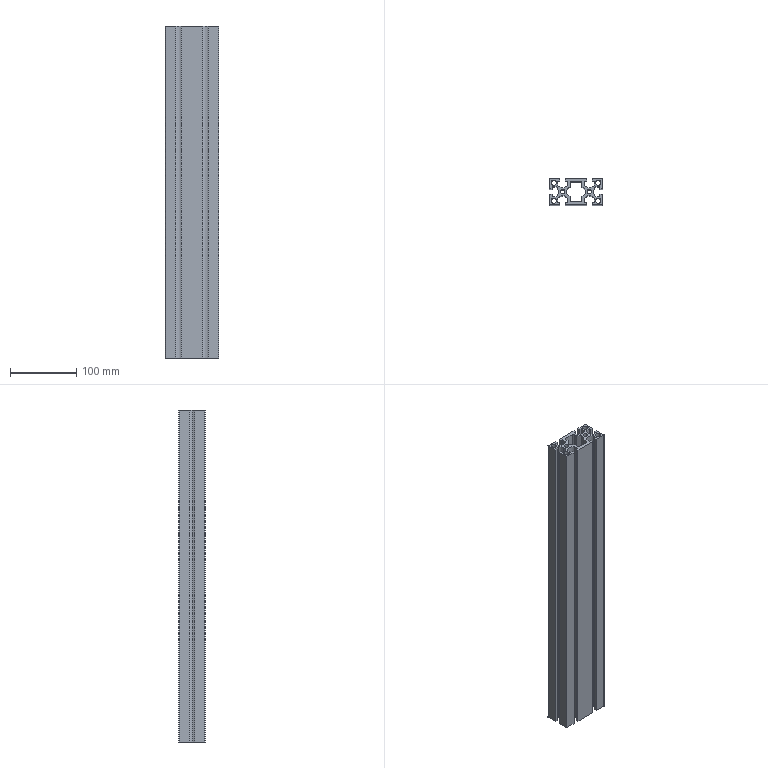Part | STEP file | 40x80 aluminium profile (L=500) | 1 solid | 87 faces | box 80 x 40 x 500 mm | volume 667060 mm3 | plane 60 | cylinder 27 | commonest cylinder face diameters 8 x8 17.549 x7 1 x4 4 x4 6.8 x4